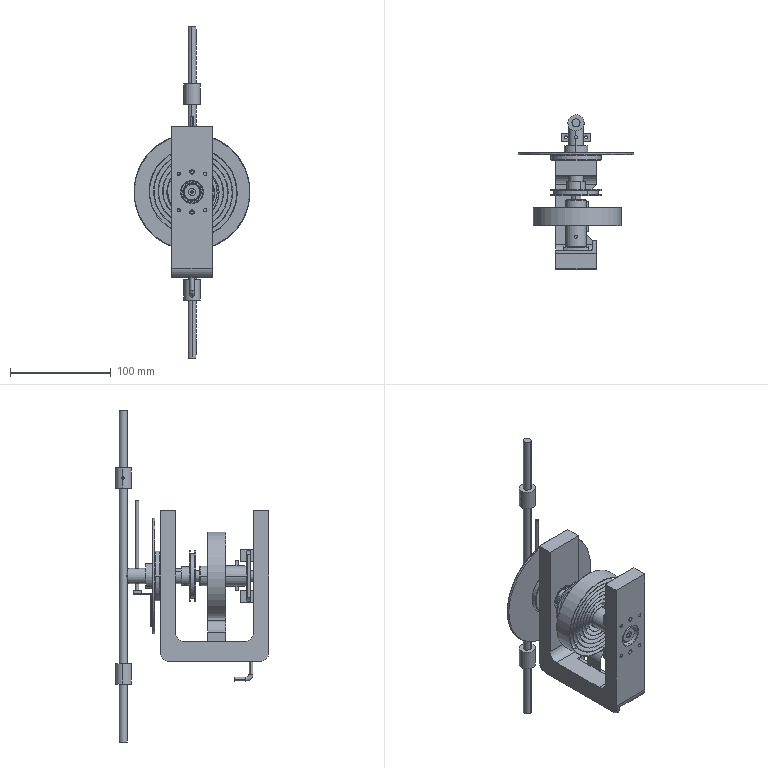Part | SolidWorks | features CompositeCurve 2 | 30 solids | 2547 faces | box 115 x 153 x 330 mm | volume 328755 mm3 | plane 1571 | cylinder 678 | sphere 148 | torus 82 | cone 66 | spline 2 | commonest cylinder face diameters 100 x288 7.8 x61 95 x37 98 x36 2.5 x28 3 x18